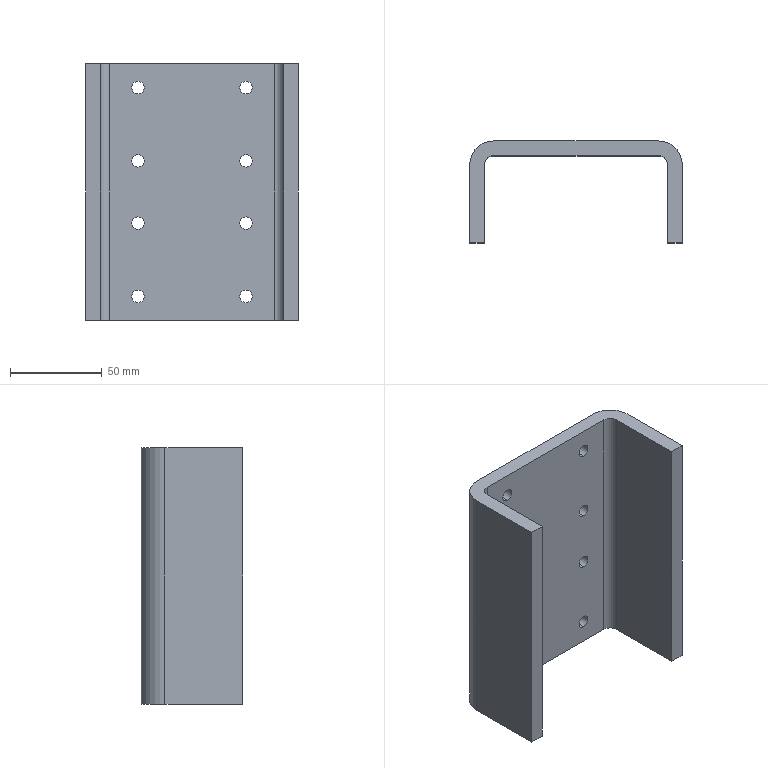Part | SolidWorks | features Extrusion 1, HoleWzd 1 | 1 solid | 30 faces | box 116 x 55.5 x 140 mm | volume 225343 mm3 | cylinder 20 | plane 10 | commonest cylinder face diameters 6.8 x16 10 x2 26 x2
STEP:
#1=CARTESIAN_POINT('',(28.5,47.5,9.6));
#2=VERTEX_POINT('',#1);
#3=CARTESIAN_POINT('',(28.5,47.5,16.4));
#4=VERTEX_POINT('',#3);
#5=CARTESIAN_POINT('',(28.5,47.5,13.));
#6=DIRECTION('',(0.,1.,0.));
#7=DIRECTION('',(0.,0.,1.));
#8=AXIS2_PLACEMENT_3D('',#5,#6,#7);
#9=CIRCLE('',#8,3.4);
#10=EDGE_CURVE('',#2,#4,#9,.T.);
#11=ORIENTED_EDGE('',*,*,#10,.F.);
#12=CARTESIAN_POINT('',(28.5,55.5,9.6));
#13=VERTEX_POINT('',#12);
#14=CARTESIAN_POINT('',(28.5,55.5,9.6));
#15=DIRECTION('',(0.,1.,0.));
#16=VECTOR('',#15,1000.);
#17=LINE('',#14,#16);
#18=EDGE_CURVE('',#2,#13,#17,.T.);
#19=ORIENTED_EDGE('',*,*,#18,.T.);
#20=CARTESIAN_POINT('',(28.5,55.5,16.4));
#21=VERTEX_POINT('',#20);
#22=CARTESIAN_POINT('',(28.5,55.5,13.));
#23=DIRECTION('',(0.,1.,0.));
#24=DIRECTION('',(0.,0.,1.));
#25=AXIS2_PLACEMENT_3D('',#22,#23,#24);
#26=CIRCLE('',#25,3.4);
#27=EDGE_CURVE('',#13,#21,#26,.T.);
#28=ORIENTED_EDGE('',*,*,#27,.T.);
#29=CARTESIAN_POINT('',(28.5,55.5,16.4));
#30=DIRECTION('',(0.,1.,0.));
#31=VECTOR('',#30,1000.);
#32=LINE('',#29,#31);
#33=EDGE_CURVE('',#4,#21,#32,.T.);
#34=ORIENTED_EDGE('',*,*,#33,.F.);
#35=EDGE_LOOP('',(#11,#19,#28,#34));
#36=FACE_OUTER_BOUND('',#35,.T.);
#37=CARTESIAN_POINT('',(28.5,55.5,13.));
#38=DIRECTION('',(0.,1.,0.));
#39=DIRECTION('',(0.,0.,1.));
#40=AXIS2_PLACEMENT_3D('',#37,#38,#39);
#41=CYLINDRICAL_SURFACE('',#40,3.4);
#42=ADVANCED_FACE('',(#36),#41,.F.);
#43=CARTESIAN_POINT('',(87.5,47.5,9.6));
#44=VERTEX_POINT('',#43);
#45=CARTESIAN_POINT('',(87.5,47.5,16.4));
#46=VERTEX_POINT('',#45);
#47=CARTESIAN_POINT('',(87.5,47.5,13.));
#48=DIRECTION('',(0.,1.,0.));
#49=DIRECTION('',(0.,0.,1.));
#50=AXIS2_PLACEMENT_3D('',#47,#48,#49);
#51=CIRCLE('',#50,3.4);
#52=EDGE_CURVE('',#44,#46,#51,.T.);
#53=ORIENTED_EDGE('',*,*,#52,.F.);
#54=CARTESIAN_POINT('',(87.5,55.5,9.6));
#55=VERTEX_POINT('',#54);
#56=CARTESIAN_POINT('',(87.5,55.5,9.6));
#57=DIRECTION('',(0.,1.,0.));
#58=VECTOR('',#57,1000.);
#59=LINE('',#56,#58);
#60=EDGE_CURVE('',#44,#55,#59,.T.);
#61=ORIENTED_EDGE('',*,*,#60,.T.);
#62=CARTESIAN_POINT('',(87.5,55.5,16.4));
#63=VERTEX_POINT('',#62);
#64=CARTESIAN_POINT('',(87.5,55.5,13.));
#65=DIRECTION('',(0.,1.,0.));
#66=DIRECTION('',(0.,0.,1.));
#67=AXIS2_PLACEMENT_3D('',#64,#65,#66);
#68=CIRCLE('',#67,3.4);
#69=EDGE_CURVE('',#55,#63,#68,.T.);
#70=ORIENTED_EDGE('',*,*,#69,.T.);
#71=CARTESIAN_POINT('',(87.5,55.5,16.4));
#72=DIRECTION('',(0.,1.,0.));
#73=VECTOR('',#72,1000.);
#74=LINE('',#71,#73);
#75=EDGE_CURVE('',#46,#63,#74,.T.);
#76=ORIENTED_EDGE('',*,*,#75,.F.);
#77=EDGE_LOOP('',(#53,#61,#70,#76));
#78=FACE_OUTER_BOUND('',#77,.T.);
#79=CARTESIAN_POINT('',(87.5,55.5,13.));
#80=DIRECTION('',(0.,1.,0.));
#81=DIRECTION('',(0.,0.,1.));
#82=AXIS2_PLACEMENT_3D('',#79,#80,#81);
#83=CYLINDRICAL_SURFACE('',#82,3.4);
#84=ADVANCED_FACE('',(#78),#83,.F.);
#85=CARTESIAN_POINT('',(87.5,47.5,49.6));
#86=VERTEX_POINT('',#85);
#87=CARTESIAN_POINT('',(87.5,47.5,56.4));
#88=VERTEX_POINT('',#87);
#89=CARTESIAN_POINT('',(87.5,47.5,53.));
#90=DIRECTION('',(0.,1.,0.));
#91=DIRECTION('',(0.,0.,1.));
#92=AXIS2_PLACEMENT_3D('',#89,#90,#91);
#93=CIRCLE('',#92,3.4);
#94=EDGE_CURVE('',#86,#88,#93,.T.);
#95=ORIENTED_EDGE('',*,*,#94,.F.);
#96=CARTESIAN_POINT('',(87.5,55.5,49.6));
#97=VERTEX_POINT('',#96);
#98=CARTESIAN_POINT('',(87.5,55.5,49.6));
#99=DIRECTION('',(0.,1.,0.));
#100=VECTOR('',#99,1000.);
#101=LINE('',#98,#100);
#102=EDGE_CURVE('',#86,#97,#101,.T.);
#103=ORIENTED_EDGE('',*,*,#102,.T.);
#104=CARTESIAN_POINT('',(87.5,55.5,56.4));
#105=VERTEX_POINT('',#104);
#106=CARTESIAN_POINT('',(87.5,55.5,53.));
#107=DIRECTION('',(0.,1.,0.));
#108=DIRECTION('',(0.,0.,1.));
#109=AXIS2_PLACEMENT_3D('',#106,#107,#108);
#110=CIRCLE('',#109,3.4);
#111=EDGE_CURVE('',#97,#105,#110,.T.);
#112=ORIENTED_EDGE('',*,*,#111,.T.);
#113=CARTESIAN_POINT('',(87.5,55.5,56.4));
#114=DIRECTION('',(0.,1.,0.));
#115=VECTOR('',#114,1000.);
#116=LINE('',#113,#115);
#117=EDGE_CURVE('',#88,#105,#116,.T.);
#118=ORIENTED_EDGE('',*,*,#117,.F.);
#119=EDGE_LOOP('',(#95,#103,#112,#118));
#120=FACE_OUTER_BOUND('',#119,.T.);
#121=CARTESIAN_POINT('',(87.5,55.5,53.));
#122=DIRECTION('',(0.,1.,0.));
#123=DIRECTION('',(0.,0.,1.));
#124=AXIS2_PLACEMENT_3D('',#121,#122,#123);
#125=CYLINDRICAL_SURFACE('',#124,3.4);
#126=ADVANCED_FACE('',(#120),#125,.F.);
#127=CARTESIAN_POINT('',(28.5,47.5,49.6));
#128=VERTEX_POINT('',#127);
#129=CARTESIAN_POINT('',(28.5,47.5,56.4));
#130=VERTEX_POINT('',#129);
#131=CARTESIAN_POINT('',(28.5,47.5,53.));
#132=DIRECTION('',(0.,1.,0.));
#133=DIRECTION('',(0.,0.,1.));
#134=AXIS2_PLACEMENT_3D('',#131,#132,#133);
#135=CIRCLE('',#134,3.4);
#136=EDGE_CURVE('',#128,#130,#135,.T.);
#137=ORIENTED_EDGE('',*,*,#136,.F.);
#138=CARTESIAN_POINT('',(28.5,55.5,49.6));
#139=VERTEX_POINT('',#138);
#140=CARTESIAN_POINT('',(28.5,55.5,49.6));
#141=DIRECTION('',(0.,1.,0.));
#142=VECTOR('',#141,1000.);
#143=LINE('',#140,#142);
#144=EDGE_CURVE('',#128,#139,#143,.T.);
#145=ORIENTED_EDGE('',*,*,#144,.T.);
#146=CARTESIAN_POINT('',(28.5,55.5,56.4));
#147=VERTEX_POINT('',#146);
#148=CARTESIAN_POINT('',(28.5,55.5,53.));
#149=DIRECTION('',(0.,1.,0.));
#150=DIRECTION('',(0.,0.,1.));
#151=AXIS2_PLACEMENT_3D('',#148,#149,#150);
#152=CIRCLE('',#151,3.4);
#153=EDGE_CURVE('',#139,#147,#152,.T.);
#154=ORIENTED_EDGE('',*,*,#153,.T.);
#155=CARTESIAN_POINT('',(28.5,55.5,56.4));
#156=DIRECTION('',(0.,1.,0.));
#157=VECTOR('',#156,1000.);
#158=LINE('',#155,#157);
#159=EDGE_CURVE('',#130,#147,#158,.T.);
#160=ORIENTED_EDGE('',*,*,#159,.F.);
#161=EDGE_LOOP('',(#137,#145,#154,#160));
#162=FACE_OUTER_BOUND('',#161,.T.);
#163=CARTESIAN_POINT('',(28.5,55.5,53.));
#164=DIRECTION('',(0.,1.,0.));
#165=DIRECTION('',(0.,0.,1.));
#166=AXIS2_PLACEMENT_3D('',#163,#164,#165);
#167=CYLINDRICAL_SURFACE('',#166,3.4);
#168=ADVANCED_FACE('',(#162),#167,.F.);
#169=CARTESIAN_POINT('',(28.5,47.5,83.6));
#170=VERTEX_POINT('',#169);
#171=CARTESIAN_POINT('',(28.5,47.5,90.4));
#172=VERTEX_POINT('',#171);
#173=CARTESIAN_POINT('',(28.5,47.5,87.));
#174=DIRECTION('',(0.,1.,0.));
#175=DIRECTION('',(0.,0.,1.));
#176=AXIS2_PLACEMENT_3D('',#173,#174,#175);
#177=CIRCLE('',#176,3.4);
#178=EDGE_CURVE('',#170,#172,#177,.T.);
#179=ORIENTED_EDGE('',*,*,#178,.F.);
#180=CARTESIAN_POINT('',(28.5,55.5,83.6));
#181=VERTEX_POINT('',#180);
#182=CARTESIAN_POINT('',(28.5,55.5,83.6));
#183=DIRECTION('',(0.,1.,0.));
#184=VECTOR('',#183,1000.);
#185=LINE('',#182,#184);
#186=EDGE_CURVE('',#170,#181,#185,.T.);
#187=ORIENTED_EDGE('',*,*,#186,.T.);
#188=CARTESIAN_POINT('',(28.5,55.5,90.4));
#189=VERTEX_POINT('',#188);
#190=CARTESIAN_POINT('',(28.5,55.5,87.));
#191=DIRECTION('',(0.,1.,0.));
#192=DIRECTION('',(0.,0.,1.));
#193=AXIS2_PLACEMENT_3D('',#190,#191,#192);
#194=CIRCLE('',#193,3.4);
#195=EDGE_CURVE('',#181,#189,#194,.T.);
#196=ORIENTED_EDGE('',*,*,#195,.T.);
#197=CARTESIAN_POINT('',(28.5,55.5,90.4));
#198=DIRECTION('',(0.,1.,0.));
#199=VECTOR('',#198,1000.);
#200=LINE('',#197,#199);
#201=EDGE_CURVE('',#172,#189,#200,.T.);
#202=ORIENTED_EDGE('',*,*,#201,.F.);
#203=EDGE_LOOP('',(#179,#187,#196,#202));
#204=FACE_OUTER_BOUND('',#203,.T.);
#205=CARTESIAN_POINT('',(28.5,55.5,87.));
#206=DIRECTION('',(0.,1.,0.));
#207=DIRECTION('',(0.,0.,1.));
#208=AXIS2_PLACEMENT_3D('',#205,#206,#207);
#209=CYLINDRICAL_SURFACE('',#208,3.4);
#210=ADVANCED_FACE('',(#204),#209,.F.);
#211=CARTESIAN_POINT('',(87.5,47.5,83.6));
#212=VERTEX_POINT('',#211);
#213=CARTESIAN_POINT('',(87.5,47.5,90.4));
#214=VERTEX_POINT('',#213);
#215=CARTESIAN_POINT('',(87.5,47.5,87.));
#216=DIRECTION('',(0.,1.,0.));
#217=DIRECTION('',(0.,0.,1.));
#218=AXIS2_PLACEMENT_3D('',#215,#216,#217);
#219=CIRCLE('',#218,3.4);
#220=EDGE_CURVE('',#212,#214,#219,.T.);
#221=ORIENTED_EDGE('',*,*,#220,.F.);
#222=CARTESIAN_POINT('',(87.5,55.5,83.6));
#223=VERTEX_POINT('',#222);
#224=CARTESIAN_POINT('',(87.5,55.5,83.6));
#225=DIRECTION('',(0.,1.,0.));
#226=VECTOR('',#225,1000.);
#227=LINE('',#224,#226);
#228=EDGE_CURVE('',#212,#223,#227,.T.);
#229=ORIENTED_EDGE('',*,*,#228,.T.);
#230=CARTESIAN_POINT('',(87.5,55.5,90.4));
#231=VERTEX_POINT('',#230);
#232=CARTESIAN_POINT('',(87.5,55.5,87.));
#233=DIRECTION('',(0.,1.,0.));
#234=DIRECTION('',(0.,0.,1.));
#235=AXIS2_PLACEMENT_3D('',#232,#233,#234);
#236=CIRCLE('',#235,3.4);
#237=EDGE_CURVE('',#223,#231,#236,.T.);
#238=ORIENTED_EDGE('',*,*,#237,.T.);
#239=CARTESIAN_POINT('',(87.5,55.5,90.4));
#240=DIRECTION('',(0.,1.,0.));
#241=VECTOR('',#240,1000.);
#242=LINE('',#239,#241);
#243=EDGE_CURVE('',#214,#231,#242,.T.);
#244=ORIENTED_EDGE('',*,*,#243,.F.);
#245=EDGE_LOOP('',(#221,#229,#238,#244));
#246=FACE_OUTER_BOUND('',#245,.T.);
#247=CARTESIAN_POINT('',(87.5,55.5,87.));
#248=DIRECTION('',(0.,1.,0.));
#249=DIRECTION('',(0.,0.,1.));
#250=AXIS2_PLACEMENT_3D('',#247,#248,#249);
#251=CYLINDRICAL_SURFACE('',#250,3.4);
#252=ADVANCED_FACE('',(#246),#251,.F.);
#253=CARTESIAN_POINT('',(87.5,47.5,123.6));
#254=VERTEX_POINT('',#253);
#255=CARTESIAN_POINT('',(87.5,47.5,130.4));
#256=VERTEX_POINT('',#255);
#257=CARTESIAN_POINT('',(87.5,47.5,127.));
#258=DIRECTION('',(0.,1.,0.));
#259=DIRECTION('',(0.,0.,1.));
#260=AXIS2_PLACEMENT_3D('',#257,#258,#259);
#261=CIRCLE('',#260,3.4);
#262=EDGE_CURVE('',#254,#256,#261,.T.);
#263=ORIENTED_EDGE('',*,*,#262,.F.);
#264=CARTESIAN_POINT('',(87.5,55.5,123.6));
#265=VERTEX_POINT('',#264);
#266=CARTESIAN_POINT('',(87.5,55.5,123.6));
#267=DIRECTION('',(0.,1.,0.));
#268=VECTOR('',#267,1000.);
#269=LINE('',#266,#268);
#270=EDGE_CURVE('',#254,#265,#269,.T.);
#271=ORIENTED_EDGE('',*,*,#270,.T.);
#272=CARTESIAN_POINT('',(87.5,55.5,130.4));
#273=VERTEX_POINT('',#272);
#274=CARTESIAN_POINT('',(87.5,55.5,127.));
#275=DIRECTION('',(0.,1.,0.));
#276=DIRECTION('',(0.,0.,1.));
#277=AXIS2_PLACEMENT_3D('',#274,#275,#276);
#278=CIRCLE('',#277,3.4);
#279=EDGE_CURVE('',#265,#273,#278,.T.);
#280=ORIENTED_EDGE('',*,*,#279,.T.);
#281=CARTESIAN_POINT('',(87.5,55.5,130.4));
#282=DIRECTION('',(0.,1.,0.));
#283=VECTOR('',#282,1000.);
#284=LINE('',#281,#283);
#285=EDGE_CURVE('',#256,#273,#284,.T.);
#286=ORIENTED_EDGE('',*,*,#285,.F.);
#287=EDGE_LOOP('',(#263,#271,#280,#286));
#288=FACE_OUTER_BOUND('',#287,.T.);
#289=CARTESIAN_POINT('',(87.5,55.5,127.));
#290=DIRECTION('',(0.,1.,0.));
#291=DIRECTION('',(0.,0.,1.));
#292=AXIS2_PLACEMENT_3D('',#289,#290,#291);
#293=CYLINDRICAL_SURFACE('',#292,3.4);
#294=ADVANCED_FACE('',(#288),#293,.F.);
#295=CARTESIAN_POINT('',(28.5,47.5,123.6));
#296=VERTEX_POINT('',#295);
#297=CARTESIAN_POINT('',(28.5,47.5,130.4));
#298=VERTEX_POINT('',#297);
#299=CARTESIAN_POINT('',(28.5,47.5,127.));
#300=DIRECTION('',(0.,1.,0.));
#301=DIRECTION('',(0.,0.,1.));
#302=AXIS2_PLACEMENT_3D('',#299,#300,#301);
#303=CIRCLE('',#302,3.4);
#304=EDGE_CURVE('',#296,#298,#303,.T.);
#305=ORIENTED_EDGE('',*,*,#304,.F.);
#306=CARTESIAN_POINT('',(28.5,55.5,123.6));
#307=VERTEX_POINT('',#306);
#308=CARTESIAN_POINT('',(28.5,55.5,123.6));
#309=DIRECTION('',(0.,1.,0.));
#310=VECTOR('',#309,1000.);
#311=LINE('',#308,#310);
#312=EDGE_CURVE('',#296,#307,#311,.T.);
#313=ORIENTED_EDGE('',*,*,#312,.T.);
#314=CARTESIAN_POINT('',(28.5,55.5,130.4));
#315=VERTEX_POINT('',#314);
#316=CARTESIAN_POINT('',(28.5,55.5,127.));
#317=DIRECTION('',(0.,1.,0.));
#318=DIRECTION('',(0.,0.,1.));
#319=AXIS2_PLACEMENT_3D('',#316,#317,#318);
#320=CIRCLE('',#319,3.4);
#321=EDGE_CURVE('',#307,#315,#320,.T.);
#322=ORIENTED_EDGE('',*,*,#321,.T.);
#323=CARTESIAN_POINT('',(28.5,55.5,130.4));
#324=DIRECTION('',(0.,1.,0.));
#325=VECTOR('',#324,1000.);
#326=LINE('',#323,#325);
#327=EDGE_CURVE('',#298,#315,#326,.T.);
#328=ORIENTED_EDGE('',*,*,#327,.F.);
#329=EDGE_LOOP('',(#305,#313,#322,#328));
#330=FACE_OUTER_BOUND('',#329,.T.);
#331=CARTESIAN_POINT('',(28.5,55.5,127.));
#332=DIRECTION('',(0.,1.,0.));
#333=DIRECTION('',(0.,0.,1.));
#334=AXIS2_PLACEMENT_3D('',#331,#332,#333);
#335=CYLINDRICAL_SURFACE('',#334,3.4);
#336=ADVANCED_FACE('',(#330),#335,.F.);
#337=CARTESIAN_POINT('',(116.,42.5,0.));
#338=VERTEX_POINT('',#337);
#339=CARTESIAN_POINT('',(116.,0.,0.));
#340=VERTEX_POINT('',#339);
#341=CARTESIAN_POINT('',(116.,42.5,0.));
#342=DIRECTION('',(0.,-1.,0.));
#343=VECTOR('',#342,1000.);
#344=LINE('',#341,#343);
#345=EDGE_CURVE('',#338,#340,#344,.T.);
#346=ORIENTED_EDGE('',*,*,#345,.F.);
#347=CARTESIAN_POINT('',(116.,42.5,140.));
#348=VERTEX_POINT('',#347);
#349=CARTESIAN_POINT('',(116.,42.5,140.));
#350=DIRECTION('',(0.,0.,-1.));
#351=VECTOR('',#350,1000.);
#352=LINE('',#349,#351);
#353=EDGE_CURVE('',#348,#338,#352,.T.);
#354=ORIENTED_EDGE('',*,*,#353,.F.);
#355=CARTESIAN_POINT('',(116.,0.,140.));
#356=VERTEX_POINT('',#355);
#357=CARTESIAN_POINT('',(116.,42.5,140.));
#358=DIRECTION('',(0.,-1.,0.));
#359=VECTOR('',#358,1000.);
#360=LINE('',#357,#359);
#361=EDGE_CURVE('',#348,#356,#360,.T.);
#362=ORIENTED_EDGE('',*,*,#361,.T.);
#363=CARTESIAN_POINT('',(116.,0.,140.));
#364=DIRECTION('',(0.,0.,-1.));
#365=VECTOR('',#364,1000.);
#366=LINE('',#363,#365);
#367=EDGE_CURVE('',#356,#340,#366,.T.);
#368=ORIENTED_EDGE('',*,*,#367,.T.);
#369=EDGE_LOOP('',(#346,#354,#362,#368));
#370=FACE_OUTER_BOUND('',#369,.T.);
#371=CARTESIAN_POINT('',(116.,42.5,140.));
#372=DIRECTION('',(1.,0.,0.));
#373=DIRECTION('',(0.,0.,-1.));
#374=AXIS2_PLACEMENT_3D('',#371,#372,#373);
#375=PLANE('',#374);
#376=ADVANCED_FACE('',(#370),#375,.T.);
#377=CARTESIAN_POINT('',(103.,55.5,0.));
#378=VERTEX_POINT('',#377);
#379=CARTESIAN_POINT('',(103.,42.5,0.));
#380=DIRECTION('',(0.,0.,-1.));
#381=DIRECTION('',(-1.,0.,0.));
#382=AXIS2_PLACEMENT_3D('',#379,#380,#381);
#383=CIRCLE('',#382,13.);
#384=EDGE_CURVE('',#378,#338,#383,.T.);
#385=ORIENTED_EDGE('',*,*,#384,.F.);
#386=CARTESIAN_POINT('',(103.,55.5,140.));
#387=VERTEX_POINT('',#386);
#388=CARTESIAN_POINT('',(103.,55.5,140.));
#389=DIRECTION('',(0.,0.,-1.));
#390=VECTOR('',#389,1000.);
#391=LINE('',#388,#390);
#392=EDGE_CURVE('',#387,#378,#391,.T.);
#393=ORIENTED_EDGE('',*,*,#392,.F.);
#394=CARTESIAN_POINT('',(103.,42.5,140.));
#395=DIRECTION('',(0.,0.,-1.));
#396=DIRECTION('',(-1.,0.,0.));
#397=AXIS2_PLACEMENT_3D('',#394,#395,#396);
#398=CIRCLE('',#397,13.);
#399=EDGE_CURVE('',#387,#348,#398,.T.);
#400=ORIENTED_EDGE('',*,*,#399,.T.);
#401=ORIENTED_EDGE('',*,*,#353,.T.);
#402=EDGE_LOOP('',(#385,#393,#400,#401));
#403=FACE_OUTER_BOUND('',#402,.T.);
#404=CARTESIAN_POINT('',(103.,42.5,140.));
#405=DIRECTION('',(0.,0.,-1.));
#406=DIRECTION('',(-1.,0.,0.));
#407=AXIS2_PLACEMENT_3D('',#404,#405,#406);
#408=CYLINDRICAL_SURFACE('',#407,13.);
#409=ADVANCED_FACE('',(#403),#408,.T.);
#410=CARTESIAN_POINT('',(28.5,55.5,13.));
#411=DIRECTION('',(0.,1.,0.));
#412=DIRECTION('',(0.,0.,1.));
#413=AXIS2_PLACEMENT_3D('',#410,#411,#412);
#414=CIRCLE('',#413,3.4);
#415=EDGE_CURVE('',#21,#13,#414,.T.);
#416=ORIENTED_EDGE('',*,*,#415,.F.);
#417=ORIENTED_EDGE('',*,*,#27,.F.);
#418=EDGE_LOOP('',(#416,#417));
#419=FACE_BOUND('',#418,.T.);
#420=CARTESIAN_POINT('',(87.5,55.5,13.));
#421=DIRECTION('',(0.,1.,0.));
#422=DIRECTION('',(0.,0.,1.));
#423=AXIS2_PLACEMENT_3D('',#420,#421,#422);
#424=CIRCLE('',#423,3.4);
#425=EDGE_CURVE('',#63,#55,#424,.T.);
#426=ORIENTED_EDGE('',*,*,#425,.F.);
#427=ORIENTED_EDGE('',*,*,#69,.F.);
#428=EDGE_LOOP('',(#426,#427));
#429=FACE_BOUND('',#428,.T.);
#430=CARTESIAN_POINT('',(87.5,55.5,53.));
#431=DIRECTION('',(0.,1.,0.));
#432=DIRECTION('',(0.,0.,1.));
#433=AXIS2_PLACEMENT_3D('',#430,#431,#432);
#434=CIRCLE('',#433,3.4);
#435=EDGE_CURVE('',#105,#97,#434,.T.);
#436=ORIENTED_EDGE('',*,*,#435,.F.);
#437=ORIENTED_EDGE('',*,*,#111,.F.);
#438=EDGE_LOOP('',(#436,#437));
#439=FACE_BOUND('',#438,.T.);
#440=CARTESIAN_POINT('',(28.5,55.5,53.));
#441=DIRECTION('',(0.,1.,0.));
#442=DIRECTION('',(0.,0.,1.));
#443=AXIS2_PLACEMENT_3D('',#440,#441,#442);
#444=CIRCLE('',#443,3.4);
#445=EDGE_CURVE('',#147,#139,#444,.T.);
#446=ORIENTED_EDGE('',*,*,#445,.F.);
#447=ORIENTED_EDGE('',*,*,#153,.F.);
#448=EDGE_LOOP('',(#446,#447));
#449=FACE_BOUND('',#448,.T.);
#450=CARTESIAN_POINT('',(28.5,55.5,87.));
#451=DIRECTION('',(0.,1.,0.));
#452=DIRECTION('',(0.,0.,1.));
#453=AXIS2_PLACEMENT_3D('',#450,#451,#452);
#454=CIRCLE('',#453,3.4);
#455=EDGE_CURVE('',#189,#181,#454,.T.);
#456=ORIENTED_EDGE('',*,*,#455,.F.);
#457=ORIENTED_EDGE('',*,*,#195,.F.);
#458=EDGE_LOOP('',(#456,#457));
#459=FACE_BOUND('',#458,.T.);
#460=CARTESIAN_POINT('',(87.5,55.5,87.));
#461=DIRECTION('',(0.,1.,0.));
#462=DIRECTION('',(0.,0.,1.));
#463=AXIS2_PLACEMENT_3D('',#460,#461,#462);
#464=CIRCLE('',#463,3.4);
#465=EDGE_CURVE('',#231,#223,#464,.T.);
#466=ORIENTED_EDGE('',*,*,#465,.F.);
#467=ORIENTED_EDGE('',*,*,#237,.F.);
#468=EDGE_LOOP('',(#466,#467));
#469=FACE_BOUND('',#468,.T.);
#470=CARTESIAN_POINT('',(87.5,55.5,127.));
#471=DIRECTION('',(0.,1.,0.));
#472=DIRECTION('',(0.,0.,1.));
#473=AXIS2_PLACEMENT_3D('',#470,#471,#472);
#474=CIRCLE('',#473,3.4);
#475=EDGE_CURVE('',#273,#265,#474,.T.);
#476=ORIENTED_EDGE('',*,*,#475,.F.);
#477=ORIENTED_EDGE('',*,*,#279,.F.);
#478=EDGE_LOOP('',(#476,#477));
#479=FACE_BOUND('',#478,.T.);
#480=CARTESIAN_POINT('',(28.5,55.5,127.));
#481=DIRECTION('',(0.,1.,0.));
#482=DIRECTION('',(0.,0.,1.));
#483=AXIS2_PLACEMENT_3D('',#480,#481,#482);
#484=CIRCLE('',#483,3.4);
#485=EDGE_CURVE('',#315,#307,#484,.T.);
#486=ORIENTED_EDGE('',*,*,#485,.F.);
#487=ORIENTED_EDGE('',*,*,#321,.F.);
#488=EDGE_LOOP('',(#486,#487));
#489=FACE_BOUND('',#488,.T.);
#490=CARTESIAN_POINT('',(13.,55.5,0.));
#491=VERTEX_POINT('',#490);
#492=CARTESIAN_POINT('',(13.,55.5,0.));
#493=DIRECTION('',(1.,0.,0.));
#494=VECTOR('',#493,1000.);
#495=LINE('',#492,#494);
#496=EDGE_CURVE('',#491,#378,#495,.T.);
#497=ORIENTED_EDGE('',*,*,#496,.F.);
#498=CARTESIAN_POINT('',(13.,55.5,140.));
#499=VERTEX_POINT('',#498);
#500=CARTESIAN_POINT('',(13.,55.5,140.));
#501=DIRECTION('',(0.,0.,-1.));
#502=VECTOR('',#501,1000.);
#503=LINE('',#500,#502);
#504=EDGE_CURVE('',#499,#491,#503,.T.);
#505=ORIENTED_EDGE('',*,*,#504,.F.);
#506=CARTESIAN_POINT('',(13.,55.5,140.));
#507=DIRECTION('',(1.,0.,0.));
#508=VECTOR('',#507,1000.);
#509=LINE('',#506,#508);
#510=EDGE_CURVE('',#499,#387,#509,.T.);
#511=ORIENTED_EDGE('',*,*,#510,.T.);
#512=ORIENTED_EDGE('',*,*,#392,.T.);
#513=EDGE_LOOP('',(#497,#505,#511,#512));
#514=FACE_OUTER_BOUND('',#513,.T.);
#515=CARTESIAN_POINT('',(13.,55.5,140.));
#516=DIRECTION('',(0.,1.,0.));
#517=DIRECTION('',(0.,0.,1.));
#518=AXIS2_PLACEMENT_3D('',#515,#516,#517);
#519=PLANE('',#518);
#520=ADVANCED_FACE('',(#419,#429,#439,#449,#459,#469,#479,#489,#514),#519,.T.);
#521=CARTESIAN_POINT('',(0.,42.5,0.));
#522=VERTEX_POINT('',#521);
#523=CARTESIAN_POINT('',(13.,42.5,0.));
#524=DIRECTION('',(0.,0.,-1.));
#525=DIRECTION('',(-1.,0.,0.));
#526=AXIS2_PLACEMENT_3D('',#523,#524,#525);
#527=CIRCLE('',#526,13.);
#528=EDGE_CURVE('',#522,#491,#527,.T.);
#529=ORIENTED_EDGE('',*,*,#528,.F.);
#530=CARTESIAN_POINT('',(0.,42.5,140.));
#531=VERTEX_POINT('',#530);
#532=CARTESIAN_POINT('',(0.,42.5,140.));
#533=DIRECTION('',(0.,0.,-1.));
#534=VECTOR('',#533,1000.);
#535=LINE('',#532,#534);
#536=EDGE_CURVE('',#531,#522,#535,.T.);
#537=ORIENTED_EDGE('',*,*,#536,.F.);
#538=CARTESIAN_POINT('',(13.,42.5,140.));
#539=DIRECTION('',(0.,0.,-1.));
#540=DIRECTION('',(-1.,0.,0.));
#541=AXIS2_PLACEMENT_3D('',#538,#539,#540);
#542=CIRCLE('',#541,13.);
#543=EDGE_CURVE('',#531,#499,#542,.T.);
#544=ORIENTED_EDGE('',*,*,#543,.T.);
#545=ORIENTED_EDGE('',*,*,#504,.T.);
#546=EDGE_LOOP('',(#529,#537,#544,#545));
#547=FACE_OUTER_BOUND('',#546,.T.);
#548=CARTESIAN_POINT('',(13.,42.5,140.));
#549=DIRECTION('',(0.,0.,-1.));
#550=DIRECTION('',(-1.,0.,0.));
#551=AXIS2_PLACEMENT_3D('',#548,#549,#550);
#552=CYLINDRICAL_SURFACE('',#551,13.);
#553=ADVANCED_FACE('',(#547),#552,.T.);
#554=CARTESIAN_POINT('',(0.,0.,0.));
#555=VERTEX_POINT('',#554);
#556=CARTESIAN_POINT('',(0.,0.,0.));
#557=DIRECTION('',(0.,1.,0.));
#558=VECTOR('',#557,1000.);
#559=LINE('',#556,#558);
#560=EDGE_CURVE('',#555,#522,#559,.T.);
#561=ORIENTED_EDGE('',*,*,#560,.F.);
#562=CARTESIAN_POINT('',(0.,0.,140.));
#563=VERTEX_POINT('',#562);
#564=CARTESIAN_POINT('',(0.,0.,140.));
#565=DIRECTION('',(0.,0.,-1.));
#566=VECTOR('',#565,1000.);
#567=LINE('',#564,#566);
#568=EDGE_CURVE('',#563,#555,#567,.T.);
#569=ORIENTED_EDGE('',*,*,#568,.F.);
#570=CARTESIAN_POINT('',(0.,0.,140.));
#571=DIRECTION('',(0.,1.,0.));
#572=VECTOR('',#571,1000.);
#573=LINE('',#570,#572);
#574=EDGE_CURVE('',#563,#531,#573,.T.);
#575=ORIENTED_EDGE('',*,*,#574,.T.);
#576=ORIENTED_EDGE('',*,*,#536,.T.);
#577=EDGE_LOOP('',(#561,#569,#575,#576));
#578=FACE_OUTER_BOUND('',#577,.T.);
#579=CARTESIAN_POINT('',(0.,0.,140.));
#580=DIRECTION('',(-1.,0.,0.));
#581=DIRECTION('',(0.,0.,1.));
#582=AXIS2_PLACEMENT_3D('',#579,#580,#581);
#583=PLANE('',#582);
#584=ADVANCED_FACE('',(#578),#583,.T.);
#585=CARTESIAN_POINT('',(8.,0.,0.));
#586=VERTEX_POINT('',#585);
#587=CARTESIAN_POINT('',(8.,0.,0.));
#588=DIRECTION('',(-1.,0.,0.));
#589=VECTOR('',#588,1000.);
#590=LINE('',#587,#589);
#591=EDGE_CURVE('',#586,#555,#590,.T.);
#592=ORIENTED_EDGE('',*,*,#591,.F.);
#593=CARTESIAN_POINT('',(8.,0.,140.));
#594=VERTEX_POINT('',#593);
#595=CARTESIAN_POINT('',(8.,0.,140.));
#596=DIRECTION('',(0.,0.,-1.));
#597=VECTOR('',#596,1000.);
#598=LINE('',#595,#597);
#599=EDGE_CURVE('',#594,#586,#598,.T.);
#600=ORIENTED_EDGE('',*,*,#599,.F.);
#601=CARTESIAN_POINT('',(8.,0.,140.));
#602=DIRECTION('',(-1.,0.,0.));
#603=VECTOR('',#602,1000.);
#604=LINE('',#601,#603);
#605=EDGE_CURVE('',#594,#563,#604,.T.);
#606=ORIENTED_EDGE('',*,*,#605,.T.);
#607=ORIENTED_EDGE('',*,*,#568,.T.);
#608=EDGE_LOOP('',(#592,#600,#606,#607));
#609=FACE_OUTER_BOUND('',#608,.T.);
#610=CARTESIAN_POINT('',(8.,0.,140.));
#611=DIRECTION('',(0.,-1.,0.));
#612=DIRECTION('',(0.,0.,-1.));
#613=AXIS2_PLACEMENT_3D('',#610,#611,#612);
#614=PLANE('',#613);
#615=ADVANCED_FACE('',(#609),#614,.T.);
#616=CARTESIAN_POINT('',(8.,42.5,0.));
#617=VERTEX_POINT('',#616);
#618=CARTESIAN_POINT('',(8.,0.,0.));
#619=DIRECTION('',(0.,1.,0.));
#620=VECTOR('',#619,1000.);
#621=LINE('',#618,#620);
#622=EDGE_CURVE('',#586,#617,#621,.T.);
#623=ORIENTED_EDGE('',*,*,#622,.T.);
#624=CARTESIAN_POINT('',(8.,42.5,140.));
#625=VERTEX_POINT('',#624);
#626=CARTESIAN_POINT('',(8.,42.5,140.));
#627=DIRECTION('',(0.,0.,-1.));
#628=VECTOR('',#627,1000.);
#629=LINE('',#626,#628);
#630=EDGE_CURVE('',#625,#617,#629,.T.);
#631=ORIENTED_EDGE('',*,*,#630,.F.);
#632=CARTESIAN_POINT('',(8.,0.,140.));
#633=DIRECTION('',(0.,1.,0.));
#634=VECTOR('',#633,1000.);
#635=LINE('',#632,#634);
#636=EDGE_CURVE('',#594,#625,#635,.T.);
#637=ORIENTED_EDGE('',*,*,#636,.F.);
#638=ORIENTED_EDGE('',*,*,#599,.T.);
#639=EDGE_LOOP('',(#623,#631,#637,#638));
#640=FACE_OUTER_BOUND('',#639,.T.);
#641=CARTESIAN_POINT('',(8.,0.,140.));
#642=DIRECTION('',(-1.,0.,0.));
#643=DIRECTION('',(0.,0.,1.));
#644=AXIS2_PLACEMENT_3D('',#641,#642,#643);
#645=PLANE('',#644);
#646=ADVANCED_FACE('',(#640),#645,.F.);
#647=CARTESIAN_POINT('',(13.,47.5,0.));
#648=VERTEX_POINT('',#647);
#649=CARTESIAN_POINT('',(13.,42.5,0.));
#650=DIRECTION('',(0.,0.,-1.));
#651=DIRECTION('',(-1.,0.,0.));
#652=AXIS2_PLACEMENT_3D('',#649,#650,#651);
#653=CIRCLE('',#652,5.);
#654=EDGE_CURVE('',#617,#648,#653,.T.);
#655=ORIENTED_EDGE('',*,*,#654,.T.);
#656=CARTESIAN_POINT('',(13.,47.5,140.));
#657=VERTEX_POINT('',#656);
#658=CARTESIAN_POINT('',(13.,47.5,140.));
#659=DIRECTION('',(0.,0.,-1.));
#660=VECTOR('',#659,1000.);
#661=LINE('',#658,#660);
#662=EDGE_CURVE('',#657,#648,#661,.T.);
#663=ORIENTED_EDGE('',*,*,#662,.F.);
#664=CARTESIAN_POINT('',(13.,42.5,140.));
#665=DIRECTION('',(0.,0.,-1.));
#666=DIRECTION('',(-1.,0.,0.));
#667=AXIS2_PLACEMENT_3D('',#664,#665,#666);
#668=CIRCLE('',#667,5.);
#669=EDGE_CURVE('',#625,#657,#668,.T.);
#670=ORIENTED_EDGE('',*,*,#669,.F.);
#671=ORIENTED_EDGE('',*,*,#630,.T.);
#672=EDGE_LOOP('',(#655,#663,#670,#671));
#673=FACE_OUTER_BOUND('',#672,.T.);
#674=CARTESIAN_POINT('',(13.,42.5,140.));
#675=DIRECTION('',(0.,0.,-1.));
#676=DIRECTION('',(-1.,0.,0.));
#677=AXIS2_PLACEMENT_3D('',#674,#675,#676);
#678=CYLINDRICAL_SURFACE('',#677,5.);
#679=ADVANCED_FACE('',(#673),#678,.F.);
#680=CARTESIAN_POINT('',(28.5,47.5,13.));
#681=DIRECTION('',(0.,1.,0.));
#682=DIRECTION('',(0.,0.,1.));
#683=AXIS2_PLACEMENT_3D('',#680,#681,#682);
#684=CIRCLE('',#683,3.4);
#685=EDGE_CURVE('',#4,#2,#684,.T.);
#686=ORIENTED_EDGE('',*,*,#685,.T.);
#687=ORIENTED_EDGE('',*,*,#10,.T.);
#688=EDGE_LOOP('',(#686,#687));
#689=FACE_BOUND('',#688,.T.);
#690=CARTESIAN_POINT('',(87.5,47.5,13.));
#691=DIRECTION('',(0.,1.,0.));
#692=DIRECTION('',(0.,0.,1.));
#693=AXIS2_PLACEMENT_3D('',#690,#691,#692);
#694=CIRCLE('',#693,3.4);
#695=EDGE_CURVE('',#46,#44,#694,.T.);
#696=ORIENTED_EDGE('',*,*,#695,.T.);
#697=ORIENTED_EDGE('',*,*,#52,.T.);
#698=EDGE_LOOP('',(#696,#697));
#699=FACE_BOUND('',#698,.T.);
#700=CARTESIAN_POINT('',(87.5,47.5,53.));
#701=DIRECTION('',(0.,1.,0.));
#702=DIRECTION('',(0.,0.,1.));
#703=AXIS2_PLACEMENT_3D('',#700,#701,#702);
#704=CIRCLE('',#703,3.4);
#705=EDGE_CURVE('',#88,#86,#704,.T.);
#706=ORIENTED_EDGE('',*,*,#705,.T.);
#707=ORIENTED_EDGE('',*,*,#94,.T.);
#708=EDGE_LOOP('',(#706,#707));
#709=FACE_BOUND('',#708,.T.);
#710=CARTESIAN_POINT('',(28.5,47.5,53.));
#711=DIRECTION('',(0.,1.,0.));
#712=DIRECTION('',(0.,0.,1.));
#713=AXIS2_PLACEMENT_3D('',#710,#711,#712);
#714=CIRCLE('',#713,3.4);
#715=EDGE_CURVE('',#130,#128,#714,.T.);
#716=ORIENTED_EDGE('',*,*,#715,.T.);
#717=ORIENTED_EDGE('',*,*,#136,.T.);
#718=EDGE_LOOP('',(#716,#717));
#719=FACE_BOUND('',#718,.T.);
#720=CARTESIAN_POINT('',(28.5,47.5,87.));
#721=DIRECTION('',(0.,1.,0.));
#722=DIRECTION('',(0.,0.,1.));
#723=AXIS2_PLACEMENT_3D('',#720,#721,#722);
#724=CIRCLE('',#723,3.4);
#725=EDGE_CURVE('',#172,#170,#724,.T.);
#726=ORIENTED_EDGE('',*,*,#725,.T.);
#727=ORIENTED_EDGE('',*,*,#178,.T.);
#728=EDGE_LOOP('',(#726,#727));
#729=FACE_BOUND('',#728,.T.);
#730=CARTESIAN_POINT('',(87.5,47.5,87.));
#731=DIRECTION('',(0.,1.,0.));
#732=DIRECTION('',(0.,0.,1.));
#733=AXIS2_PLACEMENT_3D('',#730,#731,#732);
#734=CIRCLE('',#733,3.4);
#735=EDGE_CURVE('',#214,#212,#734,.T.);
#736=ORIENTED_EDGE('',*,*,#735,.T.);
#737=ORIENTED_EDGE('',*,*,#220,.T.);
#738=EDGE_LOOP('',(#736,#737));
#739=FACE_BOUND('',#738,.T.);
#740=CARTESIAN_POINT('',(87.5,47.5,127.));
#741=DIRECTION('',(0.,1.,0.));
#742=DIRECTION('',(0.,0.,1.));
#743=AXIS2_PLACEMENT_3D('',#740,#741,#742);
#744=CIRCLE('',#743,3.4);
#745=EDGE_CURVE('',#256,#254,#744,.T.);
#746=ORIENTED_EDGE('',*,*,#745,.T.);
#747=ORIENTED_EDGE('',*,*,#262,.T.);
#748=EDGE_LOOP('',(#746,#747));
#749=FACE_BOUND('',#748,.T.);
#750=CARTESIAN_POINT('',(28.5,47.5,127.));
#751=DIRECTION('',(0.,1.,0.));
#752=DIRECTION('',(0.,0.,1.));
#753=AXIS2_PLACEMENT_3D('',#750,#751,#752);
#754=CIRCLE('',#753,3.4);
#755=EDGE_CURVE('',#298,#296,#754,.T.);
#756=ORIENTED_EDGE('',*,*,#755,.T.);
#757=ORIENTED_EDGE('',*,*,#304,.T.);
#758=EDGE_LOOP('',(#756,#757));
#759=FACE_BOUND('',#758,.T.);
#760=CARTESIAN_POINT('',(103.,47.5,0.));
#761=VERTEX_POINT('',#760);
#762=CARTESIAN_POINT('',(13.,47.5,0.));
#763=DIRECTION('',(1.,0.,0.));
#764=VECTOR('',#763,1000.);
#765=LINE('',#762,#764);
#766=EDGE_CURVE('',#648,#761,#765,.T.);
#767=ORIENTED_EDGE('',*,*,#766,.T.);
#768=CARTESIAN_POINT('',(103.,47.5,140.));
#769=VERTEX_POINT('',#768);
#770=CARTESIAN_POINT('',(103.,47.5,140.));
#771=DIRECTION('',(0.,0.,-1.));
#772=VECTOR('',#771,1000.);
#773=LINE('',#770,#772);
#774=EDGE_CURVE('',#769,#761,#773,.T.);
#775=ORIENTED_EDGE('',*,*,#774,.F.);
#776=CARTESIAN_POINT('',(13.,47.5,140.));
#777=DIRECTION('',(1.,0.,0.));
#778=VECTOR('',#777,1000.);
#779=LINE('',#776,#778);
#780=EDGE_CURVE('',#657,#769,#779,.T.);
#781=ORIENTED_EDGE('',*,*,#780,.F.);
#782=ORIENTED_EDGE('',*,*,#662,.T.);
#783=EDGE_LOOP('',(#767,#775,#781,#782));
#784=FACE_OUTER_BOUND('',#783,.T.);
#785=CARTESIAN_POINT('',(13.,47.5,140.));
#786=DIRECTION('',(0.,1.,0.));
#787=DIRECTION('',(0.,0.,1.));
#788=AXIS2_PLACEMENT_3D('',#785,#786,#787);
#789=PLANE('',#788);
#790=ADVANCED_FACE('',(#689,#699,#709,#719,#729,#739,#749,#759,#784),#789,.F.);
#791=CARTESIAN_POINT('',(108.,42.5,0.));
#792=VERTEX_POINT('',#791);
#793=CARTESIAN_POINT('',(103.,42.5,0.));
#794=DIRECTION('',(0.,0.,-1.));
#795=DIRECTION('',(-1.,0.,0.));
#796=AXIS2_PLACEMENT_3D('',#793,#794,#795);
#797=CIRCLE('',#796,5.);
#798=EDGE_CURVE('',#761,#792,#797,.T.);
#799=ORIENTED_EDGE('',*,*,#798,.T.);
#800=CARTESIAN_POINT('',(108.,42.5,140.));
#801=VERTEX_POINT('',#800);
#802=CARTESIAN_POINT('',(108.,42.5,140.));
#803=DIRECTION('',(0.,0.,-1.));
#804=VECTOR('',#803,1000.);
#805=LINE('',#802,#804);
#806=EDGE_CURVE('',#801,#792,#805,.T.);
#807=ORIENTED_EDGE('',*,*,#806,.F.);
#808=CARTESIAN_POINT('',(103.,42.5,140.));
#809=DIRECTION('',(0.,0.,-1.));
#810=DIRECTION('',(-1.,0.,0.));
#811=AXIS2_PLACEMENT_3D('',#808,#809,#810);
#812=CIRCLE('',#811,5.);
#813=EDGE_CURVE('',#769,#801,#812,.T.);
#814=ORIENTED_EDGE('',*,*,#813,.F.);
#815=ORIENTED_EDGE('',*,*,#774,.T.);
#816=EDGE_LOOP('',(#799,#807,#814,#815));
#817=FACE_OUTER_BOUND('',#816,.T.);
#818=CARTESIAN_POINT('',(103.,42.5,140.));
#819=DIRECTION('',(0.,0.,-1.));
#820=DIRECTION('',(-1.,0.,0.));
#821=AXIS2_PLACEMENT_3D('',#818,#819,#820);
#822=CYLINDRICAL_SURFACE('',#821,5.);
#823=ADVANCED_FACE('',(#817),#822,.F.);
#824=CARTESIAN_POINT('',(108.,0.,0.));
#825=VERTEX_POINT('',#824);
#826=CARTESIAN_POINT('',(108.,42.5,0.));
#827=DIRECTION('',(0.,-1.,0.));
#828=VECTOR('',#827,1000.);
#829=LINE('',#826,#828);
#830=EDGE_CURVE('',#792,#825,#829,.T.);
#831=ORIENTED_EDGE('',*,*,#830,.T.);
#832=CARTESIAN_POINT('',(108.,0.,140.));
#833=VERTEX_POINT('',#832);
#834=CARTESIAN_POINT('',(108.,0.,140.));
#835=DIRECTION('',(0.,0.,-1.));
#836=VECTOR('',#835,1000.);
#837=LINE('',#834,#836);
#838=EDGE_CURVE('',#833,#825,#837,.T.);
#839=ORIENTED_EDGE('',*,*,#838,.F.);
#840=CARTESIAN_POINT('',(108.,42.5,140.));
#841=DIRECTION('',(0.,-1.,0.));
#842=VECTOR('',#841,1000.);
#843=LINE('',#840,#842);
#844=EDGE_CURVE('',#801,#833,#843,.T.);
#845=ORIENTED_EDGE('',*,*,#844,.F.);
#846=ORIENTED_EDGE('',*,*,#806,.T.);
#847=EDGE_LOOP('',(#831,#839,#845,#846));
#848=FACE_OUTER_BOUND('',#847,.T.);
#849=CARTESIAN_POINT('',(108.,42.5,140.));
#850=DIRECTION('',(1.,0.,0.));
#851=DIRECTION('',(0.,0.,-1.));
#852=AXIS2_PLACEMENT_3D('',#849,#850,#851);
#853=PLANE('',#852);
#854=ADVANCED_FACE('',(#848),#853,.F.);
#855=CARTESIAN_POINT('',(116.,0.,0.));
#856=DIRECTION('',(-1.,0.,0.));
#857=VECTOR('',#856,1000.);
#858=LINE('',#855,#857);
#859=EDGE_CURVE('',#340,#825,#858,.T.);
#860=ORIENTED_EDGE('',*,*,#859,.F.);
#861=ORIENTED_EDGE('',*,*,#367,.F.);
#862=CARTESIAN_POINT('',(116.,0.,140.));
#863=DIRECTION('',(-1.,0.,0.));
#864=VECTOR('',#863,1000.);
#865=LINE('',#862,#864);
#866=EDGE_CURVE('',#356,#833,#865,.T.);
#867=ORIENTED_EDGE('',*,*,#866,.T.);
#868=ORIENTED_EDGE('',*,*,#838,.T.);
#869=EDGE_LOOP('',(#860,#861,#867,#868));
#870=FACE_OUTER_BOUND('',#869,.T.);
#871=CARTESIAN_POINT('',(116.,0.,140.));
#872=DIRECTION('',(0.,-1.,0.));
#873=DIRECTION('',(0.,0.,-1.));
#874=AXIS2_PLACEMENT_3D('',#871,#872,#873);
#875=PLANE('',#874);
#876=ADVANCED_FACE('',(#870),#875,.T.);
#877=ORIENTED_EDGE('',*,*,#361,.F.);
#878=ORIENTED_EDGE('',*,*,#399,.F.);
#879=ORIENTED_EDGE('',*,*,#510,.F.);
#880=ORIENTED_EDGE('',*,*,#543,.F.);
#881=ORIENTED_EDGE('',*,*,#574,.F.);
#882=ORIENTED_EDGE('',*,*,#605,.F.);
#883=ORIENTED_EDGE('',*,*,#636,.T.);
#884=ORIENTED_EDGE('',*,*,#669,.T.);
#885=ORIENTED_EDGE('',*,*,#780,.T.);
#886=ORIENTED_EDGE('',*,*,#813,.T.);
#887=ORIENTED_EDGE('',*,*,#844,.T.);
#888=ORIENTED_EDGE('',*,*,#866,.F.);
#889=EDGE_LOOP('',(#877,#878,#879,#880,#881,#882,#883,#884,#885,#886,#887,#888));
#890=FACE_OUTER_BOUND('',#889,.T.);
#891=CARTESIAN_POINT('',(103.,42.5,140.));
#892=DIRECTION('',(0.,0.,-1.));
#893=DIRECTION('',(-1.,0.,0.));
#894=AXIS2_PLACEMENT_3D('',#891,#892,#893);
#895=PLANE('',#894);
#896=ADVANCED_FACE('',(#890),#895,.F.);
#897=ORIENTED_EDGE('',*,*,#345,.T.);
#898=ORIENTED_EDGE('',*,*,#859,.T.);
#899=ORIENTED_EDGE('',*,*,#830,.F.);
#900=ORIENTED_EDGE('',*,*,#798,.F.);
#901=ORIENTED_EDGE('',*,*,#766,.F.);
#902=ORIENTED_EDGE('',*,*,#654,.F.);
#903=ORIENTED_EDGE('',*,*,#622,.F.);
#904=ORIENTED_EDGE('',*,*,#591,.T.);
#905=ORIENTED_EDGE('',*,*,#560,.T.);
#906=ORIENTED_EDGE('',*,*,#528,.T.);
#907=ORIENTED_EDGE('',*,*,#496,.T.);
#908=ORIENTED_EDGE('',*,*,#384,.T.);
#909=EDGE_LOOP('',(#897,#898,#899,#900,#901,#902,#903,#904,#905,#906,#907,#908));
#910=FACE_OUTER_BOUND('',#909,.T.);
#911=CARTESIAN_POINT('',(103.,42.5,0.));
#912=DIRECTION('',(0.,0.,-1.));
#913=DIRECTION('',(-1.,0.,0.));
#914=AXIS2_PLACEMENT_3D('',#911,#912,#913);
#915=PLANE('',#914);
#916=ADVANCED_FACE('',(#910),#915,.T.);
#917=ORIENTED_EDGE('',*,*,#312,.F.);
#918=ORIENTED_EDGE('',*,*,#755,.F.);
#919=ORIENTED_EDGE('',*,*,#327,.T.);
#920=ORIENTED_EDGE('',*,*,#485,.T.);
#921=EDGE_LOOP('',(#917,#918,#919,#920));
#922=FACE_OUTER_BOUND('',#921,.T.);
#923=CARTESIAN_POINT('',(28.5,55.5,127.));
#924=DIRECTION('',(0.,1.,0.));
#925=DIRECTION('',(0.,0.,1.));
#926=AXIS2_PLACEMENT_3D('',#923,#924,#925);
#927=CYLINDRICAL_SURFACE('',#926,3.4);
#928=ADVANCED_FACE('',(#922),#927,.F.);
#929=ORIENTED_EDGE('',*,*,#270,.F.);
#930=ORIENTED_EDGE('',*,*,#745,.F.);
#931=ORIENTED_EDGE('',*,*,#285,.T.);
#932=ORIENTED_EDGE('',*,*,#475,.T.);
#933=EDGE_LOOP('',(#929,#930,#931,#932));
#934=FACE_OUTER_BOUND('',#933,.T.);
#935=CARTESIAN_POINT('',(87.5,55.5,127.));
#936=DIRECTION('',(0.,1.,0.));
#937=DIRECTION('',(0.,0.,1.));
#938=AXIS2_PLACEMENT_3D('',#935,#936,#937);
#939=CYLINDRICAL_SURFACE('',#938,3.4);
#940=ADVANCED_FACE('',(#934),#939,.F.);
#941=ORIENTED_EDGE('',*,*,#228,.F.);
#942=ORIENTED_EDGE('',*,*,#735,.F.);
#943=ORIENTED_EDGE('',*,*,#243,.T.);
#944=ORIENTED_EDGE('',*,*,#465,.T.);
#945=EDGE_LOOP('',(#941,#942,#943,#944));
#946=FACE_OUTER_BOUND('',#945,.T.);
#947=CARTESIAN_POINT('',(87.5,55.5,87.));
#948=DIRECTION('',(0.,1.,0.));
#949=DIRECTION('',(0.,0.,1.));
#950=AXIS2_PLACEMENT_3D('',#947,#948,#949);
#951=CYLINDRICAL_SURFACE('',#950,3.4);
#952=ADVANCED_FACE('',(#946),#951,.F.);
#953=ORIENTED_EDGE('',*,*,#186,.F.);
#954=ORIENTED_EDGE('',*,*,#725,.F.);
#955=ORIENTED_EDGE('',*,*,#201,.T.);
#956=ORIENTED_EDGE('',*,*,#455,.T.);
#957=EDGE_LOOP('',(#953,#954,#955,#956));
#958=FACE_OUTER_BOUND('',#957,.T.);
#959=CARTESIAN_POINT('',(28.5,55.5,87.));
#960=DIRECTION('',(0.,1.,0.));
#961=DIRECTION('',(0.,0.,1.));
#962=AXIS2_PLACEMENT_3D('',#959,#960,#961);
#963=CYLINDRICAL_SURFACE('',#962,3.4);
#964=ADVANCED_FACE('',(#958),#963,.F.);
#965=ORIENTED_EDGE('',*,*,#144,.F.);
#966=ORIENTED_EDGE('',*,*,#715,.F.);
#967=ORIENTED_EDGE('',*,*,#159,.T.);
#968=ORIENTED_EDGE('',*,*,#445,.T.);
#969=EDGE_LOOP('',(#965,#966,#967,#968));
#970=FACE_OUTER_BOUND('',#969,.T.);
#971=CARTESIAN_POINT('',(28.5,55.5,53.));
#972=DIRECTION('',(0.,1.,0.));
#973=DIRECTION('',(0.,0.,1.));
#974=AXIS2_PLACEMENT_3D('',#971,#972,#973);
#975=CYLINDRICAL_SURFACE('',#974,3.4);
#976=ADVANCED_FACE('',(#970),#975,.F.);
#977=ORIENTED_EDGE('',*,*,#102,.F.);
#978=ORIENTED_EDGE('',*,*,#705,.F.);
#979=ORIENTED_EDGE('',*,*,#117,.T.);
#980=ORIENTED_EDGE('',*,*,#435,.T.);
#981=EDGE_LOOP('',(#977,#978,#979,#980));
#982=FACE_OUTER_BOUND('',#981,.T.);
#983=CARTESIAN_POINT('',(87.5,55.5,53.));
#984=DIRECTION('',(0.,1.,0.));
#985=DIRECTION('',(0.,0.,1.));
#986=AXIS2_PLACEMENT_3D('',#983,#984,#985);
#987=CYLINDRICAL_SURFACE('',#986,3.4);
#988=ADVANCED_FACE('',(#982),#987,.F.);
#989=ORIENTED_EDGE('',*,*,#60,.F.);
#990=ORIENTED_EDGE('',*,*,#695,.F.);
#991=ORIENTED_EDGE('',*,*,#75,.T.);
#992=ORIENTED_EDGE('',*,*,#425,.T.);
#993=EDGE_LOOP('',(#989,#990,#991,#992));
#994=FACE_OUTER_BOUND('',#993,.T.);
#995=CARTESIAN_POINT('',(87.5,55.5,13.));
#996=DIRECTION('',(0.,1.,0.));
#997=DIRECTION('',(0.,0.,1.));
#998=AXIS2_PLACEMENT_3D('',#995,#996,#997);
#999=CYLINDRICAL_SURFACE('',#998,3.4);
#1000=ADVANCED_FACE('',(#994),#999,.F.);
#1001=ORIENTED_EDGE('',*,*,#18,.F.);
#1002=ORIENTED_EDGE('',*,*,#685,.F.);
#1003=ORIENTED_EDGE('',*,*,#33,.T.);
#1004=ORIENTED_EDGE('',*,*,#415,.T.);
#1005=EDGE_LOOP('',(#1001,#1002,#1003,#1004));
#1006=FACE_OUTER_BOUND('',#1005,.T.);
#1007=CARTESIAN_POINT('',(28.5,55.5,13.));
#1008=DIRECTION('',(0.,1.,0.));
#1009=DIRECTION('',(0.,0.,1.));
#1010=AXIS2_PLACEMENT_3D('',#1007,#1008,#1009);
#1011=CYLINDRICAL_SURFACE('',#1010,3.4);
#1012=ADVANCED_FACE('',(#1006),#1011,.F.);
#1013=CLOSED_SHELL('',(#42,#84,#126,#168,#210,#252,#294,#336,#376,#409,#520,#553,#584,#615,#646,#679,#790,#823,#854,#876,#896,#916,#928,#940,#952,#964,#976,#988,#1000,#1012));
#1014=MANIFOLD_SOLID_BREP('',#1013);
#1015=CARTESIAN_POINT('',(0.,0.,0.));
#1016=DIRECTION('',(0.,0.,1.));
#1017=DIRECTION('',(1.,0.,0.));
#1018=AXIS2_PLACEMENT_3D('',#1015,#1016,#1017);
#1019=(LENGTH_UNIT()NAMED_UNIT(*)SI_UNIT(.MILLI.,.METRE.));
#1020=UNCERTAINTY_MEASURE_WITH_UNIT(LENGTH_MEASURE(0.00001),#1019,'','');
#1021=(NAMED_UNIT(*)PLANE_ANGLE_UNIT()SI_UNIT($,.RADIAN.));
#1022=(NAMED_UNIT(*)SI_UNIT($,.STERADIAN.)SOLID_ANGLE_UNIT());
#1023=(GEOMETRIC_REPRESENTATION_CONTEXT(3)GLOBAL_UNCERTAINTY_ASSIGNED_CONTEXT((#1020))GLOBAL_UNIT_ASSIGNED_CONTEXT((#1019,#1021,#1022))REPRESENTATION_CONTEXT('',''));
#1024=ADVANCED_BREP_SHAPE_REPRESENTATION('',(#1014,#1018),#1023);